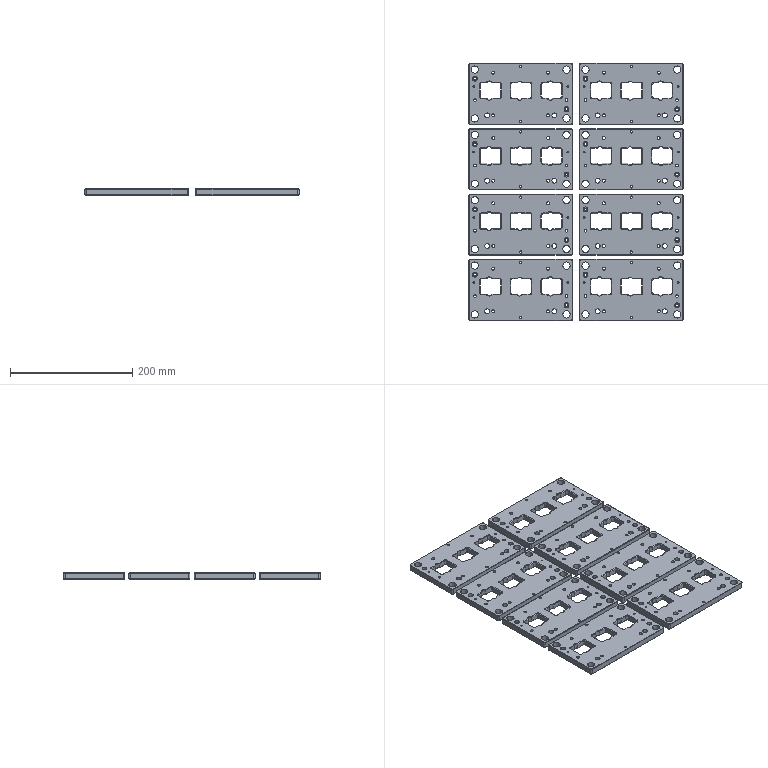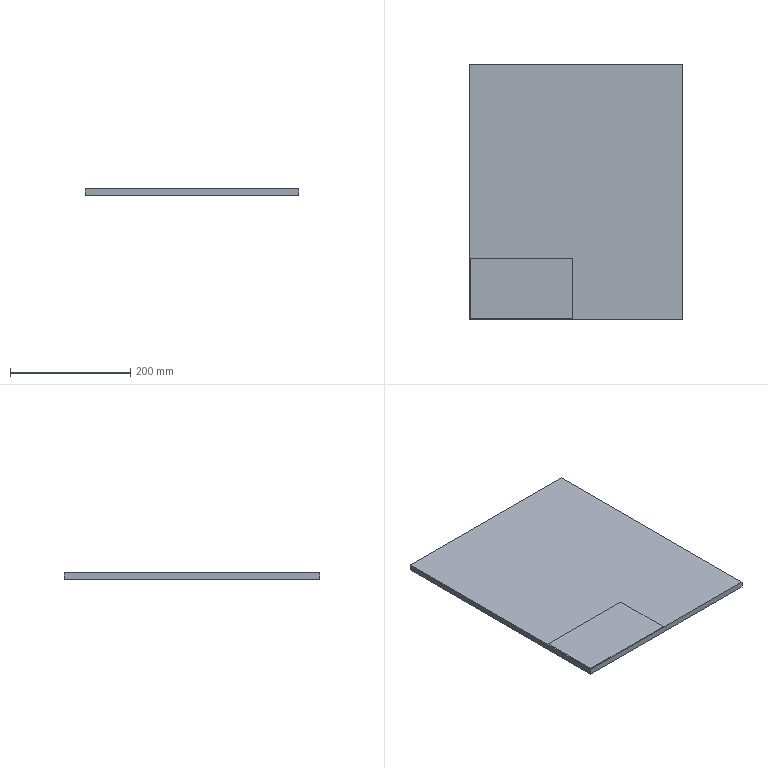CAM job | NX | 3-axis milling, drilling | part box 351 x 421 x 10 mm | stock box 355 x 425 x 10 mm
Tools:
number,name,description,diameter,corner_radius,flute_length,length,flutes
2,D4A45,Milling Tool-5 Parameters,4.0,0.0,2.0,2.0,2
6,D6,Milling Tool-5 Parameters,6.0,0.0,50.0,75.0,2
4,D4,Milling Tool-5 Parameters,4.0,0.0,50.0,75.0,2
3,D3,Milling Tool-5 Parameters,3.0,0.0,50.0,75.0,2
14,4.5ZT,Drilling Tool,4.0,0.0,35.0,50.0,2
12,2.5ZT,Drilling Tool,2.5,0.0,35.0,50.0,2
Operations:
program,operation,operation_type,tool,method,geometry_group,spindle_rpm,surface_speed,feed_per_tooth,feed_cut,feed_plunge,cut_length_mm,path_length_mm,cut_time_min,machine_time_min
1吸,ZLEVEL_PROFILE_COPY_COPY_1_COPY,ZLevelMilling,D6,METHOD,A,9500.0,179.0,0.1158,2200.0,1000.0,89367.334,91415.68,40.787,40.992
1吸,ZLEVEL_PROFILE_COPY_COPY_1_COPY_COPY,ZLevelMilling,D6,METHOD,A,9500.0,179.0,0.1158,2200.0,1000.0,47149.358,50867.86,21.928,22.3
1吸,HOLE_MILLING,CylinderMilling,D6,METHOD,A,9500.0,179.0,0.1158,2200.0,100.0,12890.58,16865.29,5.859,6.257
1吸,ZLEVEL_PROFILE_COPY_COPY_COPY,ZLevelMilling,D6,MILL_FINISH,A,9500.0,119.0,0.0632,1200.0,1000.0,2406.42,6050.761,2.015,2.379
1吸,ZLEVEL_PROFILE_COPY_COPY_1_COPY_COPY_COPY,ZLevelMilling,D3,METHOD,A,9500.0,89.0,0.0632,1200.0,1000.0,15335.478,28724.136,13.224,14.563
1吸,ZLEVEL_PROFILE_1_COPY_1_COPY,ZLevelMilling,D4A45,METHOD,A,9500.0,179.0,0.0526,1000.0,100.0,9856.173,39518.281,9.856,12.822
1吸,刀补6,CylinderMilling,D6,METHOD,A,9500.0,179.0,0.0632,1200.0,100.0,3963.508,7938.218,3.303,3.7
1吸,ZLEVEL_PROFILE_COPY_COPY_COPY_COPY,ZLevelMilling,D4,MILL_FINISH,A,9500.0,119.0,0.0632,1200.0,1000.0,4420.401,6405.098,3.687,3.885
2,DRILLING_COPY,Operation,D4A45,METHOD,B,5000.0,62.0,0.025,250.0,0.0,72.0,679.604,0.288,0.3488
2,DRILLING_COPY_COPY_COPY_COPY,Operation,4.5ZT,METHOD,B,1910.0,21.0,0.0471,180.0,0.0,62.807,395.069,0.3489,0.3822
2,DRILLING_COPY_COPY_COPY_COPY_COPY,Operation,4.5ZT,METHOD,B,1910.0,21.0,0.0471,180.0,0.0,62.807,424.792,0.3489,0.3851
2,DRILLING_COPY_COPY_COPY_COPY_COPY_COPY,Operation,2.5ZT,METHOD,B,1910.0,21.0,0.0471,180.0,0.0,30.502,278.034,0.1695,0.1942
2,HOLE_MILLING_COPY,CylinderMilling,D6,METHOD,B,9500.0,179.0,0.0789,1500.0,100.0,428.488,891.094,0.2857,0.3319
2,HOLE_MILLING_COPY_COPY,CylinderMilling,D3,METHOD,B,9500.0,89.0,0.0526,1000.0,100.0,988.54,1841.345,0.9885,1.074
2,ZLEVEL_PROFILE_1_COPY_1_COPY_COPY,ZLevelMilling,D4A45,METHOD,B,9500.0,179.0,0.0526,1000.0,100.0,1253.258,4731.267,1.253,1.601
2,刀补,CylinderMilling,D3,METHOD,B,9500.0,89.0,0.0526,1000.0,100.0,256.279,1109.084,0.2563,0.3416